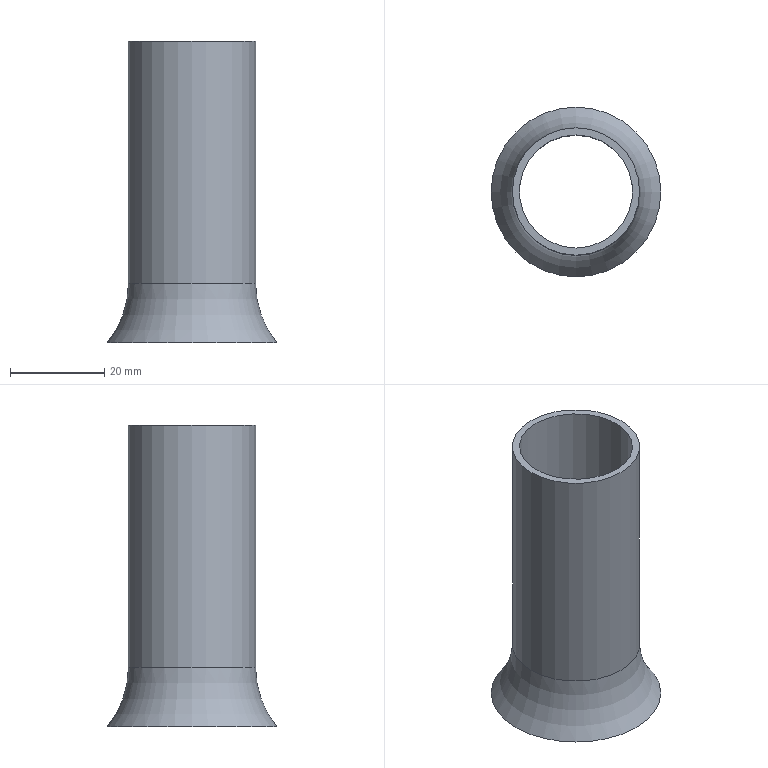Part | STEP file | 1-14.2 | 1 solid | 6 faces | box 36 x 36 x 64.039 mm | volume 7996 mm3 | torus 2 | cylinder 2 | plane 2 | commonest cylinder face diameters 24 x1 27 x1
STEP:
#1=CARTESIAN_POINT('',(0.,0.,0.));
#2=DIRECTION('',(0.,0.,1.));
#3=DIRECTION('',(1.,0.,0.));
#4=AXIS2_PLACEMENT_3D('',#1,#2,#3);
#5=CARTESIAN_POINT('',(0.,18.,-64.039));
#6=VERTEX_POINT('',#5);
#7=CARTESIAN_POINT('',(0.,0.,-64.039));
#8=DIRECTION('',(0.,0.,-1.));
#9=DIRECTION('',(0.,1.,0.));
#10=AXIS2_PLACEMENT_3D('',#7,#8,#9);
#11=CIRCLE('',#10,18.);
#12=CARTESIAN_POINT('',(0.,0.,-51.4));
#13=DIRECTION('',(0.,0.,1.));
#14=DIRECTION('',(0.,1.,0.));
#15=AXIS2_PLACEMENT_3D('',#12,#13,#14);
#16=TOROIDAL_SURFACE('',#15,33.5,20.);
#17=CARTESIAN_POINT('',(6.283,3.826));
#18=DIRECTION('',(-1.,0.));
#19=VECTOR('',#18,1.);
#20=LINE('',#17,#19);
#21=(GEOMETRIC_REPRESENTATION_CONTEXT(2)PARAMETRIC_REPRESENTATION_CONTEXT()REPRESENTATION_CONTEXT('',''));
#22=DEFINITIONAL_REPRESENTATION('',(#20),#21);
#23=PCURVE('',#16,#22);
#24=CARTESIAN_POINT('',(0.,-9.,-64.039));
#25=DIRECTION('',(0.,0.,-1.));
#26=DIRECTION('',(0.,1.,0.));
#27=AXIS2_PLACEMENT_3D('',#24,#25,#26);
#28=PLANE('',#27);
#29=CARTESIAN_POINT('',(9.,0.));
#30=DIRECTION('',(1.,0.));
#31=AXIS2_PLACEMENT_2D('',#29,#30);
#32=CIRCLE('',#31,18.);
#33=(GEOMETRIC_REPRESENTATION_CONTEXT(2)PARAMETRIC_REPRESENTATION_CONTEXT()REPRESENTATION_CONTEXT('',''));
#34=DEFINITIONAL_REPRESENTATION('',(#32),#33);
#35=PCURVE('',#28,#34);
#36=SURFACE_CURVE('',#11,(#23,#35),.PCURVE_S1.);
#37=EDGE_CURVE('',#6,#6,#36,.T.);
#38=ORIENTED_EDGE('',*,*,#37,.T.);
#39=CARTESIAN_POINT('',(0.,13.5,-51.4));
#40=VERTEX_POINT('',#39);
#41=CARTESIAN_POINT('',(0.,33.5,-51.4));
#42=DIRECTION('',(-1.,0.,0.));
#43=DIRECTION('',(0.,-0.775,-0.632));
#44=AXIS2_PLACEMENT_3D('',#41,#42,#43);
#45=CIRCLE('',#44,20.);
#46=CARTESIAN_POINT('',(0.,3.826));
#47=DIRECTION('',(0.,-1.));
#48=VECTOR('',#47,1.);
#49=LINE('',#46,#48);
#50=(GEOMETRIC_REPRESENTATION_CONTEXT(2)PARAMETRIC_REPRESENTATION_CONTEXT()REPRESENTATION_CONTEXT('',''));
#51=DEFINITIONAL_REPRESENTATION('',(#49),#50);
#52=PCURVE('',#16,#51);
#53=CARTESIAN_POINT('',(6.283,3.826));
#54=DIRECTION('',(0.,-1.));
#55=VECTOR('',#54,1.);
#56=LINE('',#53,#55);
#57=(GEOMETRIC_REPRESENTATION_CONTEXT(2)PARAMETRIC_REPRESENTATION_CONTEXT()REPRESENTATION_CONTEXT('',''));
#58=DEFINITIONAL_REPRESENTATION('',(#56),#57);
#59=PCURVE('',#16,#58);
#60=SEAM_CURVE('',#45,(#52,#59),.PCURVE_S1.);
#61=EDGE_CURVE('',#6,#40,#60,.T.);
#62=ORIENTED_EDGE('',*,*,#61,.T.);
#63=CARTESIAN_POINT('',(0.,0.,-51.4));
#64=DIRECTION('',(0.,0.,-1.));
#65=DIRECTION('',(0.,1.,0.));
#66=AXIS2_PLACEMENT_3D('',#63,#64,#65);
#67=CIRCLE('',#66,13.5);
#68=CARTESIAN_POINT('',(6.283,3.142));
#69=DIRECTION('',(-1.,0.));
#70=VECTOR('',#69,1.);
#71=LINE('',#68,#70);
#72=(GEOMETRIC_REPRESENTATION_CONTEXT(2)PARAMETRIC_REPRESENTATION_CONTEXT()REPRESENTATION_CONTEXT('',''));
#73=DEFINITIONAL_REPRESENTATION('',(#71),#72);
#74=PCURVE('',#16,#73);
#75=CARTESIAN_POINT('',(0.,0.,-51.4));
#76=DIRECTION('',(0.,0.,1.));
#77=DIRECTION('',(0.,1.,0.));
#78=AXIS2_PLACEMENT_3D('',#75,#76,#77);
#79=CYLINDRICAL_SURFACE('',#78,13.5);
#80=CARTESIAN_POINT('',(6.283,0.));
#81=DIRECTION('',(-1.,0.));
#82=VECTOR('',#81,1.);
#83=LINE('',#80,#82);
#84=(GEOMETRIC_REPRESENTATION_CONTEXT(2)PARAMETRIC_REPRESENTATION_CONTEXT()REPRESENTATION_CONTEXT('',''));
#85=DEFINITIONAL_REPRESENTATION('',(#83),#84);
#86=PCURVE('',#79,#85);
#87=SURFACE_CURVE('',#67,(#74,#86),.PCURVE_S1.);
#88=EDGE_CURVE('',#40,#40,#87,.T.);
#89=ORIENTED_EDGE('',*,*,#88,.F.);
#90=ORIENTED_EDGE('',*,*,#61,.F.);
#91=EDGE_LOOP('',(#38,#62,#89,#90));
#92=FACE_BOUND('',#91,.F.);
#93=ADVANCED_FACE('',(#92),#16,.F.);
#94=CARTESIAN_POINT('',(0.,13.5,0.));
#95=VERTEX_POINT('',#94);
#96=CARTESIAN_POINT('',(0.,13.5,-51.4));
#97=DIRECTION('',(0.,0.,1.));
#98=VECTOR('',#97,1.);
#99=LINE('',#96,#98);
#100=CARTESIAN_POINT('',(6.283,0.));
#101=DIRECTION('',(0.,1.));
#102=VECTOR('',#101,1.);
#103=LINE('',#100,#102);
#104=(GEOMETRIC_REPRESENTATION_CONTEXT(2)PARAMETRIC_REPRESENTATION_CONTEXT()REPRESENTATION_CONTEXT('',''));
#105=DEFINITIONAL_REPRESENTATION('',(#103),#104);
#106=PCURVE('',#79,#105);
#107=CARTESIAN_POINT('',(0.,0.));
#108=DIRECTION('',(0.,1.));
#109=VECTOR('',#108,1.);
#110=LINE('',#107,#109);
#111=(GEOMETRIC_REPRESENTATION_CONTEXT(2)PARAMETRIC_REPRESENTATION_CONTEXT()REPRESENTATION_CONTEXT('',''));
#112=DEFINITIONAL_REPRESENTATION('',(#110),#111);
#113=PCURVE('',#79,#112);
#114=SEAM_CURVE('',#99,(#106,#113),.PCURVE_S1.);
#115=EDGE_CURVE('',#40,#95,#114,.T.);
#116=ORIENTED_EDGE('',*,*,#115,.T.);
#117=CARTESIAN_POINT('',(0.,0.,0.));
#118=DIRECTION('',(0.,0.,-1.));
#119=DIRECTION('',(0.,1.,0.));
#120=AXIS2_PLACEMENT_3D('',#117,#118,#119);
#121=CIRCLE('',#120,13.5);
#122=CARTESIAN_POINT('',(6.283,51.4));
#123=DIRECTION('',(-1.,0.));
#124=VECTOR('',#123,1.);
#125=LINE('',#122,#124);
#126=(GEOMETRIC_REPRESENTATION_CONTEXT(2)PARAMETRIC_REPRESENTATION_CONTEXT()REPRESENTATION_CONTEXT('',''));
#127=DEFINITIONAL_REPRESENTATION('',(#125),#126);
#128=PCURVE('',#79,#127);
#129=CARTESIAN_POINT('',(0.,-6.75,0.));
#130=DIRECTION('',(0.,0.,1.));
#131=DIRECTION('',(0.,1.,0.));
#132=AXIS2_PLACEMENT_3D('',#129,#130,#131);
#133=PLANE('',#132);
#134=CARTESIAN_POINT('',(20.25,0.));
#135=CARTESIAN_POINT('',(20.25,-23.383));
#136=CARTESIAN_POINT('',(0.,-11.691));
#137=CARTESIAN_POINT('',(-20.25,0.));
#138=CARTESIAN_POINT('',(0.,11.691));
#139=CARTESIAN_POINT('',(20.25,23.383));
#140=CARTESIAN_POINT('',(20.25,0.));
#141=(BOUNDED_CURVE()B_SPLINE_CURVE(2,(#134,#135,#136,#137,#138,#139,#140),.UNSPECIFIED.,.T.,.F.)B_SPLINE_CURVE_WITH_KNOTS((1,2,2,2,2,1),(-2.094,0.,2.094,4.189,6.283,8.378),.UNSPECIFIED.)CURVE()GEOMETRIC_REPRESENTATION_ITEM()RATIONAL_B_SPLINE_CURVE((1.,0.5,1.,0.5,1.,0.5,1.))REPRESENTATION_ITEM(''));
#142=(GEOMETRIC_REPRESENTATION_CONTEXT(2)PARAMETRIC_REPRESENTATION_CONTEXT()REPRESENTATION_CONTEXT('',''));
#143=DEFINITIONAL_REPRESENTATION('',(#141),#142);
#144=PCURVE('',#133,#143);
#145=SURFACE_CURVE('',#121,(#128,#144),.PCURVE_S1.);
#146=EDGE_CURVE('',#95,#95,#145,.T.);
#147=ORIENTED_EDGE('',*,*,#146,.T.);
#148=ORIENTED_EDGE('',*,*,#115,.F.);
#149=ORIENTED_EDGE('',*,*,#88,.F.);
#150=EDGE_LOOP('',(#116,#147,#148,#149));
#151=FACE_BOUND('',#150,.T.);
#152=ADVANCED_FACE('',(#151),#79,.T.);
#153=ORIENTED_EDGE('',*,*,#146,.F.);
#154=EDGE_LOOP('',(#153));
#155=FACE_BOUND('',#154,.T.);
#156=CARTESIAN_POINT('',(0.,12.,0.));
#157=VERTEX_POINT('',#156);
#158=CARTESIAN_POINT('',(0.,0.,0.));
#159=DIRECTION('',(0.,0.,-1.));
#160=DIRECTION('',(0.,1.,0.));
#161=AXIS2_PLACEMENT_3D('',#158,#159,#160);
#162=CIRCLE('',#161,12.);
#163=CARTESIAN_POINT('',(18.75,0.));
#164=CARTESIAN_POINT('',(18.75,-20.785));
#165=CARTESIAN_POINT('',(0.75,-10.392));
#166=CARTESIAN_POINT('',(-17.25,0.));
#167=CARTESIAN_POINT('',(0.75,10.392));
#168=CARTESIAN_POINT('',(18.75,20.785));
#169=CARTESIAN_POINT('',(18.75,0.));
#170=(BOUNDED_CURVE()B_SPLINE_CURVE(2,(#163,#164,#165,#166,#167,#168,#169),.UNSPECIFIED.,.T.,.F.)B_SPLINE_CURVE_WITH_KNOTS((1,2,2,2,2,1),(-2.094,0.,2.094,4.189,6.283,8.378),.UNSPECIFIED.)CURVE()GEOMETRIC_REPRESENTATION_ITEM()RATIONAL_B_SPLINE_CURVE((1.,0.5,1.,0.5,1.,0.5,1.))REPRESENTATION_ITEM(''));
#171=(GEOMETRIC_REPRESENTATION_CONTEXT(2)PARAMETRIC_REPRESENTATION_CONTEXT()REPRESENTATION_CONTEXT('',''));
#172=DEFINITIONAL_REPRESENTATION('',(#170),#171);
#173=PCURVE('',#133,#172);
#174=CARTESIAN_POINT('',(0.,0.,-51.4));
#175=DIRECTION('',(0.,0.,1.));
#176=DIRECTION('',(0.,1.,0.));
#177=AXIS2_PLACEMENT_3D('',#174,#175,#176);
#178=CYLINDRICAL_SURFACE('',#177,12.);
#179=CARTESIAN_POINT('',(6.283,51.4));
#180=DIRECTION('',(-1.,0.));
#181=VECTOR('',#180,1.);
#182=LINE('',#179,#181);
#183=(GEOMETRIC_REPRESENTATION_CONTEXT(2)PARAMETRIC_REPRESENTATION_CONTEXT()REPRESENTATION_CONTEXT('',''));
#184=DEFINITIONAL_REPRESENTATION('',(#182),#183);
#185=PCURVE('',#178,#184);
#186=SURFACE_CURVE('',#162,(#173,#185),.PCURVE_S1.);
#187=EDGE_CURVE('',#157,#157,#186,.T.);
#188=ORIENTED_EDGE('',*,*,#187,.T.);
#189=EDGE_LOOP('',(#188));
#190=FACE_BOUND('',#189,.T.);
#191=ADVANCED_FACE('',(#155,#190),#133,.T.);
#192=ORIENTED_EDGE('',*,*,#37,.T.);
#193=EDGE_LOOP('',(#192));
#194=FACE_BOUND('',#193,.T.);
#195=CARTESIAN_POINT('',(0.,16.107,-64.039));
#196=VERTEX_POINT('',#195);
#197=CARTESIAN_POINT('',(0.,0.,-64.039));
#198=DIRECTION('',(0.,0.,-1.));
#199=DIRECTION('',(0.,1.,0.));
#200=AXIS2_PLACEMENT_3D('',#197,#198,#199);
#201=CIRCLE('',#200,16.107);
#202=CARTESIAN_POINT('',(9.,0.));
#203=DIRECTION('',(1.,0.));
#204=AXIS2_PLACEMENT_2D('',#202,#203);
#205=CIRCLE('',#204,16.107);
#206=(GEOMETRIC_REPRESENTATION_CONTEXT(2)PARAMETRIC_REPRESENTATION_CONTEXT()REPRESENTATION_CONTEXT('',''));
#207=DEFINITIONAL_REPRESENTATION('',(#205),#206);
#208=PCURVE('',#28,#207);
#209=CARTESIAN_POINT('',(0.,0.,-51.4));
#210=DIRECTION('',(0.,0.,1.));
#211=DIRECTION('',(0.,1.,0.));
#212=AXIS2_PLACEMENT_3D('',#209,#210,#211);
#213=TOROIDAL_SURFACE('',#212,33.5,21.5);
#214=CARTESIAN_POINT('',(6.283,3.77));
#215=DIRECTION('',(-1.,0.));
#216=VECTOR('',#215,1.);
#217=LINE('',#214,#216);
#218=(GEOMETRIC_REPRESENTATION_CONTEXT(2)PARAMETRIC_REPRESENTATION_CONTEXT()REPRESENTATION_CONTEXT('',''));
#219=DEFINITIONAL_REPRESENTATION('',(#217),#218);
#220=PCURVE('',#213,#219);
#221=SURFACE_CURVE('',#201,(#208,#220),.PCURVE_S1.);
#222=EDGE_CURVE('',#196,#196,#221,.T.);
#223=ORIENTED_EDGE('',*,*,#222,.F.);
#224=EDGE_LOOP('',(#223));
#225=FACE_BOUND('',#224,.T.);
#226=ADVANCED_FACE('',(#194,#225),#28,.T.);
#227=ORIENTED_EDGE('',*,*,#222,.T.);
#228=CARTESIAN_POINT('',(0.,12.,-51.4));
#229=VERTEX_POINT('',#228);
#230=CARTESIAN_POINT('',(0.,33.5,-51.4));
#231=DIRECTION('',(-1.,0.,0.));
#232=DIRECTION('',(0.,-0.809,-0.5879));
#233=AXIS2_PLACEMENT_3D('',#230,#231,#232);
#234=CIRCLE('',#233,21.5);
#235=CARTESIAN_POINT('',(0.,3.77));
#236=DIRECTION('',(0.,-1.));
#237=VECTOR('',#236,1.);
#238=LINE('',#235,#237);
#239=(GEOMETRIC_REPRESENTATION_CONTEXT(2)PARAMETRIC_REPRESENTATION_CONTEXT()REPRESENTATION_CONTEXT('',''));
#240=DEFINITIONAL_REPRESENTATION('',(#238),#239);
#241=PCURVE('',#213,#240);
#242=CARTESIAN_POINT('',(6.283,3.77));
#243=DIRECTION('',(0.,-1.));
#244=VECTOR('',#243,1.);
#245=LINE('',#242,#244);
#246=(GEOMETRIC_REPRESENTATION_CONTEXT(2)PARAMETRIC_REPRESENTATION_CONTEXT()REPRESENTATION_CONTEXT('',''));
#247=DEFINITIONAL_REPRESENTATION('',(#245),#246);
#248=PCURVE('',#213,#247);
#249=SEAM_CURVE('',#234,(#241,#248),.PCURVE_S1.);
#250=EDGE_CURVE('',#196,#229,#249,.T.);
#251=ORIENTED_EDGE('',*,*,#250,.T.);
#252=CARTESIAN_POINT('',(0.,0.,-51.4));
#253=DIRECTION('',(0.,0.,-1.));
#254=DIRECTION('',(0.,1.,0.));
#255=AXIS2_PLACEMENT_3D('',#252,#253,#254);
#256=CIRCLE('',#255,12.);
#257=CARTESIAN_POINT('',(6.283,3.142));
#258=DIRECTION('',(-1.,0.));
#259=VECTOR('',#258,1.);
#260=LINE('',#257,#259);
#261=(GEOMETRIC_REPRESENTATION_CONTEXT(2)PARAMETRIC_REPRESENTATION_CONTEXT()REPRESENTATION_CONTEXT('',''));
#262=DEFINITIONAL_REPRESENTATION('',(#260),#261);
#263=PCURVE('',#213,#262);
#264=CARTESIAN_POINT('',(6.283,0.));
#265=DIRECTION('',(-1.,0.));
#266=VECTOR('',#265,1.);
#267=LINE('',#264,#266);
#268=(GEOMETRIC_REPRESENTATION_CONTEXT(2)PARAMETRIC_REPRESENTATION_CONTEXT()REPRESENTATION_CONTEXT('',''));
#269=DEFINITIONAL_REPRESENTATION('',(#267),#268);
#270=PCURVE('',#178,#269);
#271=SURFACE_CURVE('',#256,(#263,#270),.PCURVE_S1.);
#272=EDGE_CURVE('',#229,#229,#271,.T.);
#273=ORIENTED_EDGE('',*,*,#272,.F.);
#274=ORIENTED_EDGE('',*,*,#250,.F.);
#275=EDGE_LOOP('',(#227,#251,#273,#274));
#276=FACE_BOUND('',#275,.T.);
#277=ADVANCED_FACE('',(#276),#213,.T.);
#278=CARTESIAN_POINT('',(0.,12.,-51.4));
#279=DIRECTION('',(0.,0.,1.));
#280=VECTOR('',#279,1.);
#281=LINE('',#278,#280);
#282=CARTESIAN_POINT('',(6.283,0.));
#283=DIRECTION('',(0.,1.));
#284=VECTOR('',#283,1.);
#285=LINE('',#282,#284);
#286=(GEOMETRIC_REPRESENTATION_CONTEXT(2)PARAMETRIC_REPRESENTATION_CONTEXT()REPRESENTATION_CONTEXT('',''));
#287=DEFINITIONAL_REPRESENTATION('',(#285),#286);
#288=PCURVE('',#178,#287);
#289=CARTESIAN_POINT('',(0.,0.));
#290=DIRECTION('',(0.,1.));
#291=VECTOR('',#290,1.);
#292=LINE('',#289,#291);
#293=(GEOMETRIC_REPRESENTATION_CONTEXT(2)PARAMETRIC_REPRESENTATION_CONTEXT()REPRESENTATION_CONTEXT('',''));
#294=DEFINITIONAL_REPRESENTATION('',(#292),#293);
#295=PCURVE('',#178,#294);
#296=SEAM_CURVE('',#281,(#288,#295),.PCURVE_S1.);
#297=EDGE_CURVE('',#229,#157,#296,.T.);
#298=ORIENTED_EDGE('',*,*,#297,.T.);
#299=ORIENTED_EDGE('',*,*,#187,.T.);
#300=ORIENTED_EDGE('',*,*,#297,.F.);
#301=ORIENTED_EDGE('',*,*,#272,.F.);
#302=EDGE_LOOP('',(#298,#299,#300,#301));
#303=FACE_BOUND('',#302,.F.);
#304=ADVANCED_FACE('',(#303),#178,.F.);
#305=CLOSED_SHELL('',(#93,#152,#191,#226,#277,#304));
#306=MANIFOLD_SOLID_BREP('',#305);
#307=(LENGTH_UNIT()NAMED_UNIT(*)SI_UNIT(.MILLI.,.METRE.));
#308=UNCERTAINTY_MEASURE_WITH_UNIT(LENGTH_MEASURE(0.0000001),#307,'','');
#309=(NAMED_UNIT(*)PLANE_ANGLE_UNIT()SI_UNIT($,.RADIAN.));
#310=(NAMED_UNIT(*)SI_UNIT($,.STERADIAN.)SOLID_ANGLE_UNIT());
#311=(GEOMETRIC_REPRESENTATION_CONTEXT(3)GLOBAL_UNCERTAINTY_ASSIGNED_CONTEXT((#308))GLOBAL_UNIT_ASSIGNED_CONTEXT((#307,#309,#310))REPRESENTATION_CONTEXT('',''));
#312=ADVANCED_BREP_SHAPE_REPRESENTATION('',(#4,#306),#311);